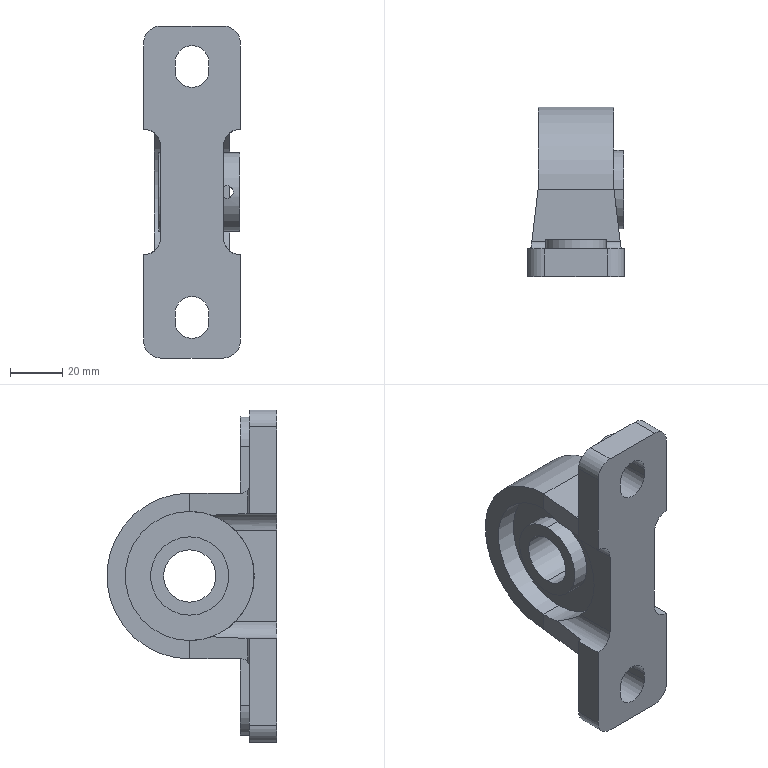Part | STEP file | T-BDJ-204 | 1 solid | 73 faces | box 37 x 65 x 127 mm | volume 102514 mm3 | cylinder 40 | plane 33 | commonest cylinder face diameters 13 x14 2 x4 4.917 x4 6 x4 30 x4 49.4 x4